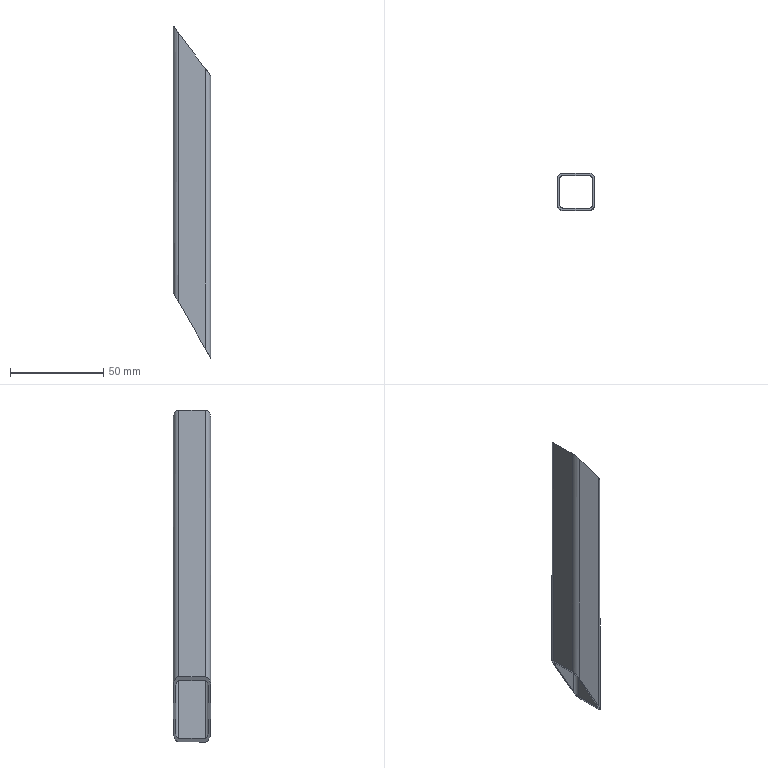Part | SolidWorks | features BaseBody 1 | 1 solid | 18 faces | box 20 x 20 x 178.414 mm | volume 12580 mm3 | plane 10 | cylinder 8 | commonest cylinder face diameters 3.6 x4 6 x4
STEP:
#1=CARTESIAN_POINT('',(10.,-7.,0.));
#2=VERTEX_POINT('',#1);
#3=CARTESIAN_POINT('',(10.,7.,0.));
#4=VERTEX_POINT('',#3);
#5=CARTESIAN_POINT('',(10.,7.,0.));
#6=DIRECTION('',(0.,1.,0.));
#7=VECTOR('',#6,1000.);
#8=LINE('',#5,#7);
#9=EDGE_CURVE('',#2,#4,#8,.T.);
#10=ORIENTED_EDGE('',*,*,#9,.T.);
#11=CARTESIAN_POINT('',(10.,7.,151.659));
#12=VERTEX_POINT('',#11);
#13=CARTESIAN_POINT('',(10.,7.,0.));
#14=DIRECTION('',(0.,0.,1.));
#15=VECTOR('',#14,1000.);
#16=LINE('',#13,#15);
#17=EDGE_CURVE('',#4,#12,#16,.T.);
#18=ORIENTED_EDGE('',*,*,#17,.T.);
#19=CARTESIAN_POINT('',(10.,-7.,151.659));
#20=VERTEX_POINT('',#19);
#21=CARTESIAN_POINT('',(10.,7.,151.659));
#22=DIRECTION('',(0.,-1.,0.));
#23=VECTOR('',#22,1000.);
#24=LINE('',#21,#23);
#25=EDGE_CURVE('',#12,#20,#24,.T.);
#26=ORIENTED_EDGE('',*,*,#25,.T.);
#27=CARTESIAN_POINT('',(10.,-7.,0.));
#28=DIRECTION('',(0.,0.,-1.));
#29=VECTOR('',#28,1000.);
#30=LINE('',#27,#29);
#31=EDGE_CURVE('',#20,#2,#30,.T.);
#32=ORIENTED_EDGE('',*,*,#31,.T.);
#33=EDGE_LOOP('',(#10,#18,#26,#32));
#34=FACE_OUTER_BOUND('',#33,.T.);
#35=CARTESIAN_POINT('',(10.,7.,0.));
#36=DIRECTION('',(1.,0.,0.));
#37=DIRECTION('',(0.,0.,-1.));
#38=AXIS2_PLACEMENT_3D('',#35,#36,#37);
#39=PLANE('',#38);
#40=ADVANCED_FACE('',(#34),#39,.T.);
#41=CARTESIAN_POINT('',(7.,10.,5.263));
#42=VERTEX_POINT('',#41);
#43=CARTESIAN_POINT('',(10.,7.,0.));
#44=CARTESIAN_POINT('',(10.,8.757,0.));
#45=CARTESIAN_POINT('',(8.757,10.,2.18));
#46=CARTESIAN_POINT('',(7.,10.,5.263));
#47=(BOUNDED_CURVE()B_SPLINE_CURVE(3,(#43,#44,#45,#46),.UNSPECIFIED.,.F.,.F.)B_SPLINE_CURVE_WITH_KNOTS((4,4),(3.142,4.712),.UNSPECIFIED.)CURVE()GEOMETRIC_REPRESENTATION_ITEM()RATIONAL_B_SPLINE_CURVE((1.,0.8047,0.8047,1.))REPRESENTATION_ITEM(''));
#48=EDGE_CURVE('',#4,#42,#47,.T.);
#49=ORIENTED_EDGE('',*,*,#48,.T.);
#50=CARTESIAN_POINT('',(7.,10.,155.672));
#51=VERTEX_POINT('',#50);
#52=CARTESIAN_POINT('',(7.,10.,0.));
#53=DIRECTION('',(0.,0.,1.));
#54=VECTOR('',#53,1000.);
#55=LINE('',#52,#54);
#56=EDGE_CURVE('',#42,#51,#55,.T.);
#57=ORIENTED_EDGE('',*,*,#56,.T.);
#58=CARTESIAN_POINT('',(7.,10.,155.672));
#59=CARTESIAN_POINT('',(8.757,10.,153.321));
#60=CARTESIAN_POINT('',(10.,8.757,151.659));
#61=CARTESIAN_POINT('',(10.,7.,151.659));
#62=(BOUNDED_CURVE()B_SPLINE_CURVE(3,(#58,#59,#60,#61),.UNSPECIFIED.,.F.,.F.)B_SPLINE_CURVE_WITH_KNOTS((4,4),(1.571,3.142),.UNSPECIFIED.)CURVE()GEOMETRIC_REPRESENTATION_ITEM()RATIONAL_B_SPLINE_CURVE((1.,0.8047,0.8047,1.))REPRESENTATION_ITEM(''));
#63=EDGE_CURVE('',#51,#12,#62,.T.);
#64=ORIENTED_EDGE('',*,*,#63,.T.);
#65=ORIENTED_EDGE('',*,*,#17,.F.);
#66=EDGE_LOOP('',(#49,#57,#64,#65));
#67=FACE_OUTER_BOUND('',#66,.T.);
#68=CARTESIAN_POINT('',(7.,7.,0.));
#69=DIRECTION('',(0.,0.,1.));
#70=DIRECTION('',(1.,0.,0.));
#71=AXIS2_PLACEMENT_3D('',#68,#69,#70);
#72=CYLINDRICAL_SURFACE('',#71,3.);
#73=ADVANCED_FACE('',(#67),#72,.T.);
#74=CARTESIAN_POINT('',(8.8,-7.,2.105));
#75=VERTEX_POINT('',#74);
#76=CARTESIAN_POINT('',(7.,-8.8,5.263));
#77=VERTEX_POINT('',#76);
#78=CARTESIAN_POINT('',(8.8,-7.,2.105));
#79=CARTESIAN_POINT('',(8.8,-8.054,2.105));
#80=CARTESIAN_POINT('',(8.054,-8.8,3.413));
#81=CARTESIAN_POINT('',(7.,-8.8,5.263));
#82=(BOUNDED_CURVE()B_SPLINE_CURVE(3,(#78,#79,#80,#81),.UNSPECIFIED.,.F.,.F.)B_SPLINE_CURVE_WITH_KNOTS((4,4),(3.142,4.712),.UNSPECIFIED.)CURVE()GEOMETRIC_REPRESENTATION_ITEM()RATIONAL_B_SPLINE_CURVE((1.,0.8047,0.8047,1.))REPRESENTATION_ITEM(''));
#83=EDGE_CURVE('',#75,#77,#82,.T.);
#84=ORIENTED_EDGE('',*,*,#83,.F.);
#85=CARTESIAN_POINT('',(8.8,7.,2.105));
#86=VERTEX_POINT('',#85);
#87=CARTESIAN_POINT('',(8.8,0.,2.105));
#88=DIRECTION('',(0.,-1.,0.));
#89=VECTOR('',#88,1000.);
#90=LINE('',#87,#89);
#91=EDGE_CURVE('',#86,#75,#90,.T.);
#92=ORIENTED_EDGE('',*,*,#91,.F.);
#93=CARTESIAN_POINT('',(7.,8.8,5.263));
#94=VERTEX_POINT('',#93);
#95=CARTESIAN_POINT('',(7.,8.8,5.263));
#96=CARTESIAN_POINT('',(8.054,8.8,3.413));
#97=CARTESIAN_POINT('',(8.8,8.054,2.105));
#98=CARTESIAN_POINT('',(8.8,7.,2.105));
#99=(BOUNDED_CURVE()B_SPLINE_CURVE(3,(#95,#96,#97,#98),.UNSPECIFIED.,.F.,.F.)B_SPLINE_CURVE_WITH_KNOTS((4,4),(1.571,3.142),.UNSPECIFIED.)CURVE()GEOMETRIC_REPRESENTATION_ITEM()RATIONAL_B_SPLINE_CURVE((1.,0.8047,0.8047,1.))REPRESENTATION_ITEM(''));
#100=EDGE_CURVE('',#94,#86,#99,.T.);
#101=ORIENTED_EDGE('',*,*,#100,.F.);
#102=CARTESIAN_POINT('',(-7.,8.8,29.825));
#103=VERTEX_POINT('',#102);
#104=CARTESIAN_POINT('',(7.548,8.8,4.302));
#105=DIRECTION('',(0.4952,0.,-0.8688));
#106=VECTOR('',#105,1000.);
#107=LINE('',#104,#106);
#108=EDGE_CURVE('',#103,#94,#107,.T.);
#109=ORIENTED_EDGE('',*,*,#108,.F.);
#110=CARTESIAN_POINT('',(-8.8,7.,32.983));
#111=VERTEX_POINT('',#110);
#112=CARTESIAN_POINT('',(-8.8,7.,32.983));
#113=CARTESIAN_POINT('',(-8.8,8.054,32.983));
#114=CARTESIAN_POINT('',(-8.054,8.8,31.675));
#115=CARTESIAN_POINT('',(-7.,8.8,29.825));
#116=(BOUNDED_CURVE()B_SPLINE_CURVE(3,(#112,#113,#114,#115),.UNSPECIFIED.,.F.,.F.)B_SPLINE_CURVE_WITH_KNOTS((4,4),(0.,1.571),.UNSPECIFIED.)CURVE()GEOMETRIC_REPRESENTATION_ITEM()RATIONAL_B_SPLINE_CURVE((1.,0.8047,0.8047,1.))REPRESENTATION_ITEM(''));
#117=EDGE_CURVE('',#111,#103,#116,.T.);
#118=ORIENTED_EDGE('',*,*,#117,.F.);
#119=CARTESIAN_POINT('',(-8.8,-7.,32.983));
#120=VERTEX_POINT('',#119);
#121=CARTESIAN_POINT('',(-8.8,0.,32.983));
#122=DIRECTION('',(0.,1.,0.));
#123=VECTOR('',#122,1000.);
#124=LINE('',#121,#123);
#125=EDGE_CURVE('',#120,#111,#124,.T.);
#126=ORIENTED_EDGE('',*,*,#125,.F.);
#127=CARTESIAN_POINT('',(-7.,-8.8,29.825));
#128=VERTEX_POINT('',#127);
#129=CARTESIAN_POINT('',(-7.,-8.8,29.825));
#130=CARTESIAN_POINT('',(-8.054,-8.8,31.675));
#131=CARTESIAN_POINT('',(-8.8,-8.054,32.983));
#132=CARTESIAN_POINT('',(-8.8,-7.,32.983));
#133=(BOUNDED_CURVE()B_SPLINE_CURVE(3,(#129,#130,#131,#132),.UNSPECIFIED.,.F.,.F.)B_SPLINE_CURVE_WITH_KNOTS((4,4),(4.712,6.283),.UNSPECIFIED.)CURVE()GEOMETRIC_REPRESENTATION_ITEM()RATIONAL_B_SPLINE_CURVE((1.,0.8047,0.8047,1.))REPRESENTATION_ITEM(''));
#134=EDGE_CURVE('',#128,#120,#133,.T.);
#135=ORIENTED_EDGE('',*,*,#134,.F.);
#136=CARTESIAN_POINT('',(7.548,-8.8,4.302));
#137=DIRECTION('',(-0.4952,0.,0.8688));
#138=VECTOR('',#137,1000.);
#139=LINE('',#136,#138);
#140=EDGE_CURVE('',#77,#128,#139,.T.);
#141=ORIENTED_EDGE('',*,*,#140,.F.);
#142=EDGE_LOOP('',(#84,#92,#101,#109,#118,#126,#135,#141));
#143=FACE_BOUND('',#142,.T.);
#144=CARTESIAN_POINT('',(7.,-10.,5.263));
#145=VERTEX_POINT('',#144);
#146=CARTESIAN_POINT('',(7.,-10.,5.263));
#147=CARTESIAN_POINT('',(8.757,-10.,2.18));
#148=CARTESIAN_POINT('',(10.,-8.757,0.));
#149=CARTESIAN_POINT('',(10.,-7.,0.));
#150=(BOUNDED_CURVE()B_SPLINE_CURVE(3,(#146,#147,#148,#149),.UNSPECIFIED.,.F.,.T.)B_SPLINE_CURVE_WITH_KNOTS((4,4),(1.571,3.142),.UNSPECIFIED.)CURVE()GEOMETRIC_REPRESENTATION_ITEM()RATIONAL_B_SPLINE_CURVE((1.,0.8047,0.8047,1.))REPRESENTATION_ITEM(''));
#151=EDGE_CURVE('',#145,#2,#150,.T.);
#152=ORIENTED_EDGE('',*,*,#151,.F.);
#153=CARTESIAN_POINT('',(-7.,-10.,29.825));
#154=VERTEX_POINT('',#153);
#155=CARTESIAN_POINT('',(7.548,-10.,4.302));
#156=DIRECTION('',(0.4952,0.,-0.8688));
#157=VECTOR('',#156,1000.);
#158=LINE('',#155,#157);
#159=EDGE_CURVE('',#154,#145,#158,.T.);
#160=ORIENTED_EDGE('',*,*,#159,.F.);
#161=CARTESIAN_POINT('',(-10.,-7.,35.088));
#162=VERTEX_POINT('',#161);
#163=CARTESIAN_POINT('',(-10.,-7.,35.088));
#164=CARTESIAN_POINT('',(-10.,-8.757,35.088));
#165=CARTESIAN_POINT('',(-8.757,-10.,32.908));
#166=CARTESIAN_POINT('',(-7.,-10.,29.825));
#167=(BOUNDED_CURVE()B_SPLINE_CURVE(3,(#163,#164,#165,#166),.UNSPECIFIED.,.F.,.F.)B_SPLINE_CURVE_WITH_KNOTS((4,4),(0.,1.571),.UNSPECIFIED.)CURVE()GEOMETRIC_REPRESENTATION_ITEM()RATIONAL_B_SPLINE_CURVE((1.,0.8047,0.8047,1.))REPRESENTATION_ITEM(''));
#168=EDGE_CURVE('',#162,#154,#167,.T.);
#169=ORIENTED_EDGE('',*,*,#168,.F.);
#170=CARTESIAN_POINT('',(-10.,7.,35.088));
#171=VERTEX_POINT('',#170);
#172=CARTESIAN_POINT('',(-10.,0.,35.088));
#173=DIRECTION('',(0.,-1.,0.));
#174=VECTOR('',#173,1000.);
#175=LINE('',#172,#174);
#176=EDGE_CURVE('',#171,#162,#175,.T.);
#177=ORIENTED_EDGE('',*,*,#176,.F.);
#178=CARTESIAN_POINT('',(-7.,10.,29.825));
#179=VERTEX_POINT('',#178);
#180=CARTESIAN_POINT('',(-7.,10.,29.825));
#181=CARTESIAN_POINT('',(-8.757,10.,32.908));
#182=CARTESIAN_POINT('',(-10.,8.757,35.088));
#183=CARTESIAN_POINT('',(-10.,7.,35.088));
#184=(BOUNDED_CURVE()B_SPLINE_CURVE(3,(#180,#181,#182,#183),.UNSPECIFIED.,.F.,.F.)B_SPLINE_CURVE_WITH_KNOTS((4,4),(4.712,6.283),.UNSPECIFIED.)CURVE()GEOMETRIC_REPRESENTATION_ITEM()RATIONAL_B_SPLINE_CURVE((1.,0.8047,0.8047,1.))REPRESENTATION_ITEM(''));
#185=EDGE_CURVE('',#179,#171,#184,.T.);
#186=ORIENTED_EDGE('',*,*,#185,.F.);
#187=CARTESIAN_POINT('',(7.548,10.,4.302));
#188=DIRECTION('',(-0.4952,0.,0.8688));
#189=VECTOR('',#188,1000.);
#190=LINE('',#187,#189);
#191=EDGE_CURVE('',#42,#179,#190,.T.);
#192=ORIENTED_EDGE('',*,*,#191,.F.);
#193=ORIENTED_EDGE('',*,*,#48,.F.);
#194=ORIENTED_EDGE('',*,*,#9,.F.);
#195=EDGE_LOOP('',(#152,#160,#169,#177,#186,#192,#193,#194));
#196=FACE_OUTER_BOUND('',#195,.T.);
#197=CARTESIAN_POINT('',(7.548,0.,4.302));
#198=DIRECTION('',(0.8688,0.,0.4952));
#199=DIRECTION('',(0.4952,0.,-0.8688));
#200=AXIS2_PLACEMENT_3D('',#197,#198,#199);
#201=PLANE('',#200);
#202=ADVANCED_FACE('',(#143,#196),#201,.F.);
#203=ORIENTED_EDGE('',*,*,#151,.T.);
#204=ORIENTED_EDGE('',*,*,#31,.F.);
#205=CARTESIAN_POINT('',(7.,-10.,155.672));
#206=VERTEX_POINT('',#205);
#207=CARTESIAN_POINT('',(10.,-7.,151.659));
#208=CARTESIAN_POINT('',(10.,-8.757,151.659));
#209=CARTESIAN_POINT('',(8.757,-10.,153.321));
#210=CARTESIAN_POINT('',(7.,-10.,155.672));
#211=(BOUNDED_CURVE()B_SPLINE_CURVE(3,(#207,#208,#209,#210),.UNSPECIFIED.,.F.,.F.)B_SPLINE_CURVE_WITH_KNOTS((4,4),(3.142,4.712),.UNSPECIFIED.)CURVE()GEOMETRIC_REPRESENTATION_ITEM()RATIONAL_B_SPLINE_CURVE((1.,0.8047,0.8047,1.))REPRESENTATION_ITEM(''));
#212=EDGE_CURVE('',#20,#206,#211,.T.);
#213=ORIENTED_EDGE('',*,*,#212,.T.);
#214=CARTESIAN_POINT('',(7.,-10.,0.));
#215=DIRECTION('',(0.,0.,-1.));
#216=VECTOR('',#215,1000.);
#217=LINE('',#214,#216);
#218=EDGE_CURVE('',#206,#145,#217,.T.);
#219=ORIENTED_EDGE('',*,*,#218,.T.);
#220=EDGE_LOOP('',(#203,#204,#213,#219));
#221=FACE_OUTER_BOUND('',#220,.T.);
#222=CARTESIAN_POINT('',(7.,-7.,0.));
#223=DIRECTION('',(0.,0.,1.));
#224=DIRECTION('',(1.,0.,0.));
#225=AXIS2_PLACEMENT_3D('',#222,#223,#224);
#226=CYLINDRICAL_SURFACE('',#225,3.);
#227=ADVANCED_FACE('',(#221),#226,.T.);
#228=CARTESIAN_POINT('',(8.8,7.,153.264));
#229=VERTEX_POINT('',#228);
#230=CARTESIAN_POINT('',(7.,8.8,155.672));
#231=VERTEX_POINT('',#230);
#232=CARTESIAN_POINT('',(8.8,7.,153.264));
#233=CARTESIAN_POINT('',(8.8,8.054,153.264));
#234=CARTESIAN_POINT('',(8.054,8.8,154.262));
#235=CARTESIAN_POINT('',(7.,8.8,155.672));
#236=(BOUNDED_CURVE()B_SPLINE_CURVE(3,(#232,#233,#234,#235),.UNSPECIFIED.,.F.,.F.)B_SPLINE_CURVE_WITH_KNOTS((4,4),(3.142,4.712),.UNSPECIFIED.)CURVE()GEOMETRIC_REPRESENTATION_ITEM()RATIONAL_B_SPLINE_CURVE((1.,0.8047,0.8047,1.))REPRESENTATION_ITEM(''));
#237=EDGE_CURVE('',#229,#231,#236,.T.);
#238=ORIENTED_EDGE('',*,*,#237,.F.);
#239=CARTESIAN_POINT('',(8.8,-7.,153.264));
#240=VERTEX_POINT('',#239);
#241=CARTESIAN_POINT('',(8.8,0.,153.264));
#242=DIRECTION('',(0.,1.,0.));
#243=VECTOR('',#242,1000.);
#244=LINE('',#241,#243);
#245=EDGE_CURVE('',#240,#229,#244,.T.);
#246=ORIENTED_EDGE('',*,*,#245,.F.);
#247=CARTESIAN_POINT('',(7.,-8.8,155.672));
#248=VERTEX_POINT('',#247);
#249=CARTESIAN_POINT('',(7.,-8.8,155.672));
#250=CARTESIAN_POINT('',(8.054,-8.8,154.262));
#251=CARTESIAN_POINT('',(8.8,-8.054,153.264));
#252=CARTESIAN_POINT('',(8.8,-7.,153.264));
#253=(BOUNDED_CURVE()B_SPLINE_CURVE(3,(#249,#250,#251,#252),.UNSPECIFIED.,.F.,.F.)B_SPLINE_CURVE_WITH_KNOTS((4,4),(1.571,3.142),.UNSPECIFIED.)CURVE()GEOMETRIC_REPRESENTATION_ITEM()RATIONAL_B_SPLINE_CURVE((1.,0.8047,0.8047,1.))REPRESENTATION_ITEM(''));
#254=EDGE_CURVE('',#248,#240,#253,.T.);
#255=ORIENTED_EDGE('',*,*,#254,.F.);
#256=CARTESIAN_POINT('',(-7.,-8.8,174.4));
#257=VERTEX_POINT('',#256);
#258=CARTESIAN_POINT('',(79.144,-8.8,59.163));
#259=DIRECTION('',(0.5987,0.,-0.8009));
#260=VECTOR('',#259,1000.);
#261=LINE('',#258,#260);
#262=EDGE_CURVE('',#257,#248,#261,.T.);
#263=ORIENTED_EDGE('',*,*,#262,.F.);
#264=CARTESIAN_POINT('',(-8.8,-7.,176.808));
#265=VERTEX_POINT('',#264);
#266=CARTESIAN_POINT('',(-8.8,-7.,176.808));
#267=CARTESIAN_POINT('',(-8.8,-8.054,176.808));
#268=CARTESIAN_POINT('',(-8.054,-8.8,175.811));
#269=CARTESIAN_POINT('',(-7.,-8.8,174.4));
#270=(BOUNDED_CURVE()B_SPLINE_CURVE(3,(#266,#267,#268,#269),.UNSPECIFIED.,.F.,.F.)B_SPLINE_CURVE_WITH_KNOTS((4,4),(0.,1.571),.UNSPECIFIED.)CURVE()GEOMETRIC_REPRESENTATION_ITEM()RATIONAL_B_SPLINE_CURVE((1.,0.8047,0.8047,1.))REPRESENTATION_ITEM(''));
#271=EDGE_CURVE('',#265,#257,#270,.T.);
#272=ORIENTED_EDGE('',*,*,#271,.F.);
#273=CARTESIAN_POINT('',(-8.8,7.,176.808));
#274=VERTEX_POINT('',#273);
#275=CARTESIAN_POINT('',(-8.8,0.,176.808));
#276=DIRECTION('',(0.,-1.,0.));
#277=VECTOR('',#276,1000.);
#278=LINE('',#275,#277);
#279=EDGE_CURVE('',#274,#265,#278,.T.);
#280=ORIENTED_EDGE('',*,*,#279,.F.);
#281=CARTESIAN_POINT('',(-7.,8.8,174.4));
#282=VERTEX_POINT('',#281);
#283=CARTESIAN_POINT('',(-7.,8.8,174.4));
#284=CARTESIAN_POINT('',(-8.054,8.8,175.811));
#285=CARTESIAN_POINT('',(-8.8,8.054,176.808));
#286=CARTESIAN_POINT('',(-8.8,7.,176.808));
#287=(BOUNDED_CURVE()B_SPLINE_CURVE(3,(#283,#284,#285,#286),.UNSPECIFIED.,.F.,.F.)B_SPLINE_CURVE_WITH_KNOTS((4,4),(4.712,6.283),.UNSPECIFIED.)CURVE()GEOMETRIC_REPRESENTATION_ITEM()RATIONAL_B_SPLINE_CURVE((1.,0.8047,0.8047,1.))REPRESENTATION_ITEM(''));
#288=EDGE_CURVE('',#282,#274,#287,.T.);
#289=ORIENTED_EDGE('',*,*,#288,.F.);
#290=CARTESIAN_POINT('',(79.144,8.8,59.163));
#291=DIRECTION('',(-0.5987,0.,0.8009));
#292=VECTOR('',#291,1000.);
#293=LINE('',#290,#292);
#294=EDGE_CURVE('',#231,#282,#293,.T.);
#295=ORIENTED_EDGE('',*,*,#294,.F.);
#296=EDGE_LOOP('',(#238,#246,#255,#263,#272,#280,#289,#295));
#297=FACE_BOUND('',#296,.T.);
#298=CARTESIAN_POINT('',(-7.,-10.,174.4));
#299=VERTEX_POINT('',#298);
#300=CARTESIAN_POINT('',(-10.,-7.,178.414));
#301=VERTEX_POINT('',#300);
#302=CARTESIAN_POINT('',(-7.,-10.,174.4));
#303=CARTESIAN_POINT('',(-8.757,-10.,176.751));
#304=CARTESIAN_POINT('',(-10.,-8.757,178.414));
#305=CARTESIAN_POINT('',(-10.,-7.,178.414));
#306=(BOUNDED_CURVE()B_SPLINE_CURVE(3,(#302,#303,#304,#305),.UNSPECIFIED.,.F.,.F.)B_SPLINE_CURVE_WITH_KNOTS((4,4),(4.712,6.283),.UNSPECIFIED.)CURVE()GEOMETRIC_REPRESENTATION_ITEM()RATIONAL_B_SPLINE_CURVE((1.,0.8047,0.8047,1.))REPRESENTATION_ITEM(''));
#307=EDGE_CURVE('',#299,#301,#306,.T.);
#308=ORIENTED_EDGE('',*,*,#307,.F.);
#309=CARTESIAN_POINT('',(79.144,-10.,59.163));
#310=DIRECTION('',(-0.5987,0.,0.8009));
#311=VECTOR('',#310,1000.);
#312=LINE('',#309,#311);
#313=EDGE_CURVE('',#206,#299,#312,.T.);
#314=ORIENTED_EDGE('',*,*,#313,.F.);
#315=ORIENTED_EDGE('',*,*,#212,.F.);
#316=ORIENTED_EDGE('',*,*,#25,.F.);
#317=ORIENTED_EDGE('',*,*,#63,.F.);
#318=CARTESIAN_POINT('',(-7.,10.,174.4));
#319=VERTEX_POINT('',#318);
#320=CARTESIAN_POINT('',(79.144,10.,59.163));
#321=DIRECTION('',(0.5987,0.,-0.8009));
#322=VECTOR('',#321,1000.);
#323=LINE('',#320,#322);
#324=EDGE_CURVE('',#319,#51,#323,.T.);
#325=ORIENTED_EDGE('',*,*,#324,.F.);
#326=CARTESIAN_POINT('',(-10.,7.,178.414));
#327=VERTEX_POINT('',#326);
#328=CARTESIAN_POINT('',(-10.,7.,178.414));
#329=CARTESIAN_POINT('',(-10.,8.757,178.414));
#330=CARTESIAN_POINT('',(-8.757,10.,176.751));
#331=CARTESIAN_POINT('',(-7.,10.,174.4));
#332=(BOUNDED_CURVE()B_SPLINE_CURVE(3,(#328,#329,#330,#331),.UNSPECIFIED.,.F.,.F.)B_SPLINE_CURVE_WITH_KNOTS((4,4),(0.,1.571),.UNSPECIFIED.)CURVE()GEOMETRIC_REPRESENTATION_ITEM()RATIONAL_B_SPLINE_CURVE((1.,0.8047,0.8047,1.))REPRESENTATION_ITEM(''));
#333=EDGE_CURVE('',#327,#319,#332,.T.);
#334=ORIENTED_EDGE('',*,*,#333,.F.);
#335=CARTESIAN_POINT('',(-10.,0.,178.414));
#336=DIRECTION('',(0.,1.,0.));
#337=VECTOR('',#336,1000.);
#338=LINE('',#335,#337);
#339=EDGE_CURVE('',#301,#327,#338,.T.);
#340=ORIENTED_EDGE('',*,*,#339,.F.);
#341=EDGE_LOOP('',(#308,#314,#315,#316,#317,#325,#334,#340));
#342=FACE_OUTER_BOUND('',#341,.T.);
#343=CARTESIAN_POINT('',(79.144,0.,59.163));
#344=DIRECTION('',(-0.8009,0.,-0.5987));
#345=DIRECTION('',(-0.5987,0.,0.8009));
#346=AXIS2_PLACEMENT_3D('',#343,#344,#345);
#347=PLANE('',#346);
#348=ADVANCED_FACE('',(#297,#342),#347,.F.);
#349=ORIENTED_EDGE('',*,*,#191,.T.);
#350=CARTESIAN_POINT('',(-7.,10.,0.));
#351=DIRECTION('',(0.,0.,1.));
#352=VECTOR('',#351,1000.);
#353=LINE('',#350,#352);
#354=EDGE_CURVE('',#179,#319,#353,.T.);
#355=ORIENTED_EDGE('',*,*,#354,.T.);
#356=ORIENTED_EDGE('',*,*,#324,.T.);
#357=ORIENTED_EDGE('',*,*,#56,.F.);
#358=EDGE_LOOP('',(#349,#355,#356,#357));
#359=FACE_OUTER_BOUND('',#358,.T.);
#360=CARTESIAN_POINT('',(-7.,10.,0.));
#361=DIRECTION('',(0.,1.,0.));
#362=DIRECTION('',(-1.,0.,0.));
#363=AXIS2_PLACEMENT_3D('',#360,#361,#362);
#364=PLANE('',#363);
#365=ADVANCED_FACE('',(#359),#364,.T.);
#366=CARTESIAN_POINT('',(7.,-8.8,0.));
#367=DIRECTION('',(0.,0.,1.));
#368=VECTOR('',#367,1000.);
#369=LINE('',#366,#368);
#370=EDGE_CURVE('',#77,#248,#369,.T.);
#371=ORIENTED_EDGE('',*,*,#370,.F.);
#372=ORIENTED_EDGE('',*,*,#140,.T.);
#373=CARTESIAN_POINT('',(-7.,-8.8,0.));
#374=DIRECTION('',(0.,0.,-1.));
#375=VECTOR('',#374,1000.);
#376=LINE('',#373,#375);
#377=EDGE_CURVE('',#257,#128,#376,.T.);
#378=ORIENTED_EDGE('',*,*,#377,.F.);
#379=ORIENTED_EDGE('',*,*,#262,.T.);
#380=EDGE_LOOP('',(#371,#372,#378,#379));
#381=FACE_OUTER_BOUND('',#380,.T.);
#382=CARTESIAN_POINT('',(7.,-8.8,0.));
#383=DIRECTION('',(0.,-1.,0.));
#384=DIRECTION('',(1.,0.,0.));
#385=AXIS2_PLACEMENT_3D('',#382,#383,#384);
#386=PLANE('',#385);
#387=ADVANCED_FACE('',(#381),#386,.F.);
#388=CARTESIAN_POINT('',(8.8,-7.,0.));
#389=DIRECTION('',(0.,0.,1.));
#390=VECTOR('',#389,1000.);
#391=LINE('',#388,#390);
#392=EDGE_CURVE('',#75,#240,#391,.T.);
#393=ORIENTED_EDGE('',*,*,#392,.F.);
#394=ORIENTED_EDGE('',*,*,#83,.T.);
#395=ORIENTED_EDGE('',*,*,#370,.T.);
#396=ORIENTED_EDGE('',*,*,#254,.T.);
#397=EDGE_LOOP('',(#393,#394,#395,#396));
#398=FACE_OUTER_BOUND('',#397,.T.);
#399=CARTESIAN_POINT('',(7.,-7.,0.));
#400=DIRECTION('',(0.,0.,1.));
#401=DIRECTION('',(1.,0.,0.));
#402=AXIS2_PLACEMENT_3D('',#399,#400,#401);
#403=CYLINDRICAL_SURFACE('',#402,1.8);
#404=ADVANCED_FACE('',(#398),#403,.F.);
#405=CARTESIAN_POINT('',(8.8,7.,0.));
#406=DIRECTION('',(0.,0.,1.));
#407=VECTOR('',#406,1000.);
#408=LINE('',#405,#407);
#409=EDGE_CURVE('',#86,#229,#408,.T.);
#410=ORIENTED_EDGE('',*,*,#409,.F.);
#411=ORIENTED_EDGE('',*,*,#91,.T.);
#412=ORIENTED_EDGE('',*,*,#392,.T.);
#413=ORIENTED_EDGE('',*,*,#245,.T.);
#414=EDGE_LOOP('',(#410,#411,#412,#413));
#415=FACE_OUTER_BOUND('',#414,.T.);
#416=CARTESIAN_POINT('',(8.8,7.,0.));
#417=DIRECTION('',(1.,0.,0.));
#418=DIRECTION('',(0.,0.,-1.));
#419=AXIS2_PLACEMENT_3D('',#416,#417,#418);
#420=PLANE('',#419);
#421=ADVANCED_FACE('',(#415),#420,.F.);
#422=CARTESIAN_POINT('',(7.,8.8,0.));
#423=DIRECTION('',(0.,0.,1.));
#424=VECTOR('',#423,1000.);
#425=LINE('',#422,#424);
#426=EDGE_CURVE('',#94,#231,#425,.T.);
#427=ORIENTED_EDGE('',*,*,#426,.F.);
#428=ORIENTED_EDGE('',*,*,#100,.T.);
#429=ORIENTED_EDGE('',*,*,#409,.T.);
#430=ORIENTED_EDGE('',*,*,#237,.T.);
#431=EDGE_LOOP('',(#427,#428,#429,#430));
#432=FACE_OUTER_BOUND('',#431,.T.);
#433=CARTESIAN_POINT('',(7.,7.,0.));
#434=DIRECTION('',(0.,0.,1.));
#435=DIRECTION('',(1.,0.,0.));
#436=AXIS2_PLACEMENT_3D('',#433,#434,#435);
#437=CYLINDRICAL_SURFACE('',#436,1.8);
#438=ADVANCED_FACE('',(#432),#437,.F.);
#439=CARTESIAN_POINT('',(-7.,8.8,0.));
#440=DIRECTION('',(0.,0.,1.));
#441=VECTOR('',#440,1000.);
#442=LINE('',#439,#441);
#443=EDGE_CURVE('',#103,#282,#442,.T.);
#444=ORIENTED_EDGE('',*,*,#443,.F.);
#445=ORIENTED_EDGE('',*,*,#108,.T.);
#446=ORIENTED_EDGE('',*,*,#426,.T.);
#447=ORIENTED_EDGE('',*,*,#294,.T.);
#448=EDGE_LOOP('',(#444,#445,#446,#447));
#449=FACE_OUTER_BOUND('',#448,.T.);
#450=CARTESIAN_POINT('',(-7.,8.8,0.));
#451=DIRECTION('',(0.,1.,0.));
#452=DIRECTION('',(-1.,0.,0.));
#453=AXIS2_PLACEMENT_3D('',#450,#451,#452);
#454=PLANE('',#453);
#455=ADVANCED_FACE('',(#449),#454,.F.);
#456=CARTESIAN_POINT('',(-8.8,7.,0.));
#457=DIRECTION('',(0.,0.,1.));
#458=VECTOR('',#457,1000.);
#459=LINE('',#456,#458);
#460=EDGE_CURVE('',#111,#274,#459,.T.);
#461=ORIENTED_EDGE('',*,*,#460,.F.);
#462=ORIENTED_EDGE('',*,*,#117,.T.);
#463=ORIENTED_EDGE('',*,*,#443,.T.);
#464=ORIENTED_EDGE('',*,*,#288,.T.);
#465=EDGE_LOOP('',(#461,#462,#463,#464));
#466=FACE_OUTER_BOUND('',#465,.T.);
#467=CARTESIAN_POINT('',(-7.,7.,0.));
#468=DIRECTION('',(0.,0.,1.));
#469=DIRECTION('',(1.,0.,0.));
#470=AXIS2_PLACEMENT_3D('',#467,#468,#469);
#471=CYLINDRICAL_SURFACE('',#470,1.8);
#472=ADVANCED_FACE('',(#466),#471,.F.);
#473=CARTESIAN_POINT('',(-8.8,-7.,0.));
#474=DIRECTION('',(0.,0.,1.));
#475=VECTOR('',#474,1000.);
#476=LINE('',#473,#475);
#477=EDGE_CURVE('',#120,#265,#476,.T.);
#478=ORIENTED_EDGE('',*,*,#477,.F.);
#479=ORIENTED_EDGE('',*,*,#125,.T.);
#480=ORIENTED_EDGE('',*,*,#460,.T.);
#481=ORIENTED_EDGE('',*,*,#279,.T.);
#482=EDGE_LOOP('',(#478,#479,#480,#481));
#483=FACE_OUTER_BOUND('',#482,.T.);
#484=CARTESIAN_POINT('',(-8.8,-7.,0.));
#485=DIRECTION('',(-1.,0.,0.));
#486=DIRECTION('',(0.,-1.,0.));
#487=AXIS2_PLACEMENT_3D('',#484,#485,#486);
#488=PLANE('',#487);
#489=ADVANCED_FACE('',(#483),#488,.F.);
#490=ORIENTED_EDGE('',*,*,#377,.T.);
#491=ORIENTED_EDGE('',*,*,#134,.T.);
#492=ORIENTED_EDGE('',*,*,#477,.T.);
#493=ORIENTED_EDGE('',*,*,#271,.T.);
#494=EDGE_LOOP('',(#490,#491,#492,#493));
#495=FACE_OUTER_BOUND('',#494,.T.);
#496=CARTESIAN_POINT('',(-7.,-7.,0.));
#497=DIRECTION('',(0.,0.,1.));
#498=DIRECTION('',(1.,0.,0.));
#499=AXIS2_PLACEMENT_3D('',#496,#497,#498);
#500=CYLINDRICAL_SURFACE('',#499,1.8);
#501=ADVANCED_FACE('',(#495),#500,.F.);
#502=ORIENTED_EDGE('',*,*,#159,.T.);
#503=ORIENTED_EDGE('',*,*,#218,.F.);
#504=ORIENTED_EDGE('',*,*,#313,.T.);
#505=CARTESIAN_POINT('',(-7.,-10.,0.));
#506=DIRECTION('',(0.,0.,-1.));
#507=VECTOR('',#506,1000.);
#508=LINE('',#505,#507);
#509=EDGE_CURVE('',#299,#154,#508,.T.);
#510=ORIENTED_EDGE('',*,*,#509,.T.);
#511=EDGE_LOOP('',(#502,#503,#504,#510));
#512=FACE_OUTER_BOUND('',#511,.T.);
#513=CARTESIAN_POINT('',(7.,-10.,0.));
#514=DIRECTION('',(0.,-1.,0.));
#515=DIRECTION('',(1.,0.,0.));
#516=AXIS2_PLACEMENT_3D('',#513,#514,#515);
#517=PLANE('',#516);
#518=ADVANCED_FACE('',(#512),#517,.T.);
#519=ORIENTED_EDGE('',*,*,#168,.T.);
#520=ORIENTED_EDGE('',*,*,#509,.F.);
#521=ORIENTED_EDGE('',*,*,#307,.T.);
#522=CARTESIAN_POINT('',(-10.,-7.,0.));
#523=DIRECTION('',(0.,0.,-1.));
#524=VECTOR('',#523,1000.);
#525=LINE('',#522,#524);
#526=EDGE_CURVE('',#301,#162,#525,.T.);
#527=ORIENTED_EDGE('',*,*,#526,.T.);
#528=EDGE_LOOP('',(#519,#520,#521,#527));
#529=FACE_OUTER_BOUND('',#528,.T.);
#530=CARTESIAN_POINT('',(-7.,-7.,0.));
#531=DIRECTION('',(0.,0.,1.));
#532=DIRECTION('',(1.,0.,0.));
#533=AXIS2_PLACEMENT_3D('',#530,#531,#532);
#534=CYLINDRICAL_SURFACE('',#533,3.);
#535=ADVANCED_FACE('',(#529),#534,.T.);
#536=ORIENTED_EDGE('',*,*,#339,.T.);
#537=CARTESIAN_POINT('',(-10.,7.,0.));
#538=DIRECTION('',(0.,0.,-1.));
#539=VECTOR('',#538,1000.);
#540=LINE('',#537,#539);
#541=EDGE_CURVE('',#327,#171,#540,.T.);
#542=ORIENTED_EDGE('',*,*,#541,.T.);
#543=ORIENTED_EDGE('',*,*,#176,.T.);
#544=ORIENTED_EDGE('',*,*,#526,.F.);
#545=EDGE_LOOP('',(#536,#542,#543,#544));
#546=FACE_OUTER_BOUND('',#545,.T.);
#547=CARTESIAN_POINT('',(-10.,-7.,0.));
#548=DIRECTION('',(-1.,0.,0.));
#549=DIRECTION('',(0.,-1.,0.));
#550=AXIS2_PLACEMENT_3D('',#547,#548,#549);
#551=PLANE('',#550);
#552=ADVANCED_FACE('',(#546),#551,.T.);
#553=ORIENTED_EDGE('',*,*,#185,.T.);
#554=ORIENTED_EDGE('',*,*,#541,.F.);
#555=ORIENTED_EDGE('',*,*,#333,.T.);
#556=ORIENTED_EDGE('',*,*,#354,.F.);
#557=EDGE_LOOP('',(#553,#554,#555,#556));
#558=FACE_OUTER_BOUND('',#557,.T.);
#559=CARTESIAN_POINT('',(-7.,7.,0.));
#560=DIRECTION('',(0.,0.,1.));
#561=DIRECTION('',(1.,0.,0.));
#562=AXIS2_PLACEMENT_3D('',#559,#560,#561);
#563=CYLINDRICAL_SURFACE('',#562,3.);
#564=ADVANCED_FACE('',(#558),#563,.T.);
#565=CLOSED_SHELL('',(#40,#73,#202,#227,#348,#365,#387,#404,#421,#438,#455,#472,#489,#501,#518,#535,#552,#564));
#566=MANIFOLD_SOLID_BREP('',#565);
#567=CARTESIAN_POINT('',(0.,0.,0.));
#568=DIRECTION('',(0.,0.,1.));
#569=DIRECTION('',(1.,0.,0.));
#570=AXIS2_PLACEMENT_3D('',#567,#568,#569);
#571=(LENGTH_UNIT()NAMED_UNIT(*)SI_UNIT(.MILLI.,.METRE.));
#572=UNCERTAINTY_MEASURE_WITH_UNIT(LENGTH_MEASURE(0.00001),#571,'','');
#573=(NAMED_UNIT(*)PLANE_ANGLE_UNIT()SI_UNIT($,.RADIAN.));
#574=(NAMED_UNIT(*)SI_UNIT($,.STERADIAN.)SOLID_ANGLE_UNIT());
#575=(GEOMETRIC_REPRESENTATION_CONTEXT(3)GLOBAL_UNCERTAINTY_ASSIGNED_CONTEXT((#572))GLOBAL_UNIT_ASSIGNED_CONTEXT((#571,#573,#574))REPRESENTATION_CONTEXT('',''));
#576=ADVANCED_BREP_SHAPE_REPRESENTATION('',(#566,#570),#575);